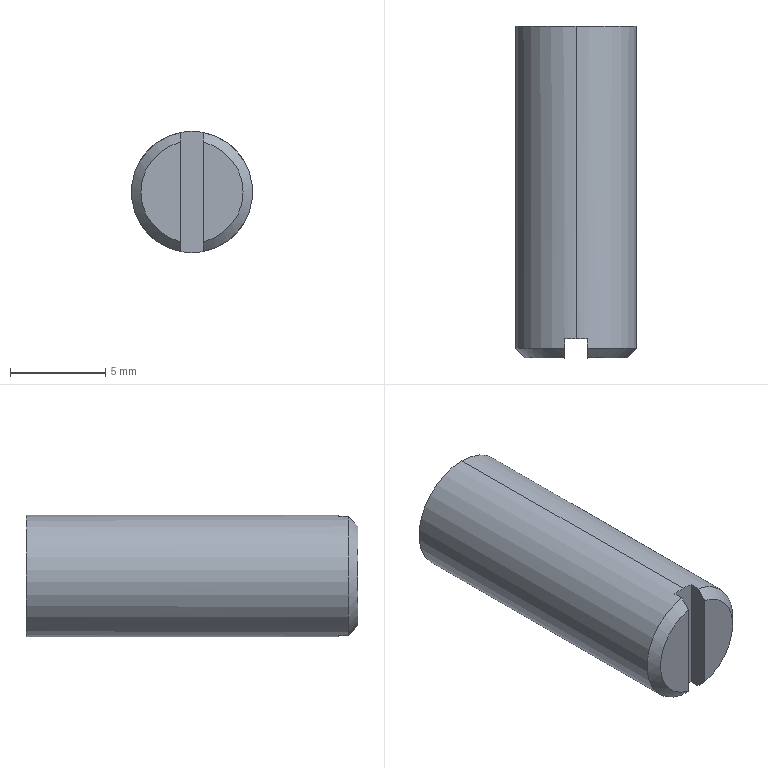Part | STEP file | 4-20.sldasm-Part-200 | 1 solid | 10 faces | box 6.35 x 17.375 x 6.35 mm | volume 540.618 mm3 | plane 6 | cylinder 2 | cone 2 | commonest cylinder face diameters 6.35 x2
STEP:
#1=CARTESIAN_POINT('',(-190.695,-588.425,-111.175));
#2=VERTEX_POINT('',#1);
#3=CARTESIAN_POINT('',(-190.695,-588.425,-104.825));
#4=VERTEX_POINT('',#3);
#5=CARTESIAN_POINT('',(-190.695,-588.425,-108.));
#6=DIRECTION('',(0.,-1.,0.));
#7=DIRECTION('',(0.,0.,-1.));
#8=AXIS2_PLACEMENT_3D('',#5,#6,#7);
#9=CIRCLE('',#8,3.175);
#10=EDGE_CURVE('',#2,#4,#9,.T.);
#11=ORIENTED_EDGE('',*,*,#10,.T.);
#12=CARTESIAN_POINT('',(-190.695,-604.8,-104.825));
#13=VERTEX_POINT('',#12);
#14=CARTESIAN_POINT('',(-190.695,-588.425,-104.825));
#15=DIRECTION('',(0.,-1.,0.));
#16=VECTOR('',#15,1000.);
#17=LINE('',#14,#16);
#18=EDGE_CURVE('',#4,#13,#17,.T.);
#19=ORIENTED_EDGE('',*,*,#18,.T.);
#20=CARTESIAN_POINT('',(-190.095,-604.8,-104.882));
#21=VERTEX_POINT('',#20);
#22=CARTESIAN_POINT('',(-190.695,-604.8,-108.));
#23=DIRECTION('',(0.,-1.,0.));
#24=DIRECTION('',(0.,0.,1.));
#25=AXIS2_PLACEMENT_3D('',#22,#23,#24);
#26=CIRCLE('',#25,3.175);
#27=EDGE_CURVE('',#21,#13,#26,.T.);
#28=ORIENTED_EDGE('',*,*,#27,.F.);
#29=CARTESIAN_POINT('',(-190.095,-605.3,-104.882));
#30=VERTEX_POINT('',#29);
#31=CARTESIAN_POINT('',(-190.095,-588.425,-104.882));
#32=DIRECTION('',(0.,1.,0.));
#33=VECTOR('',#32,1000.);
#34=LINE('',#31,#33);
#35=EDGE_CURVE('',#30,#21,#34,.T.);
#36=ORIENTED_EDGE('',*,*,#35,.F.);
#37=CARTESIAN_POINT('',(-190.095,-605.3,-111.118));
#38=VERTEX_POINT('',#37);
#39=CARTESIAN_POINT('',(-190.695,-605.3,-108.));
#40=DIRECTION('',(0.,1.,0.));
#41=DIRECTION('',(0.,0.,-1.));
#42=AXIS2_PLACEMENT_3D('',#39,#40,#41);
#43=CIRCLE('',#42,3.175);
#44=EDGE_CURVE('',#30,#38,#43,.T.);
#45=ORIENTED_EDGE('',*,*,#44,.T.);
#46=CARTESIAN_POINT('',(-190.095,-604.8,-111.118));
#47=VERTEX_POINT('',#46);
#48=CARTESIAN_POINT('',(-190.095,-588.425,-111.118));
#49=DIRECTION('',(0.,-1.,0.));
#50=VECTOR('',#49,1000.);
#51=LINE('',#48,#50);
#52=EDGE_CURVE('',#47,#38,#51,.T.);
#53=ORIENTED_EDGE('',*,*,#52,.F.);
#54=CARTESIAN_POINT('',(-190.695,-604.8,-111.175));
#55=VERTEX_POINT('',#54);
#56=CARTESIAN_POINT('',(-190.695,-604.8,-108.));
#57=DIRECTION('',(0.,-1.,0.));
#58=DIRECTION('',(0.,0.,1.));
#59=AXIS2_PLACEMENT_3D('',#56,#57,#58);
#60=CIRCLE('',#59,3.175);
#61=EDGE_CURVE('',#55,#47,#60,.T.);
#62=ORIENTED_EDGE('',*,*,#61,.F.);
#63=CARTESIAN_POINT('',(-190.695,-588.425,-111.175));
#64=DIRECTION('',(0.,-1.,0.));
#65=VECTOR('',#64,1000.);
#66=LINE('',#63,#65);
#67=EDGE_CURVE('',#2,#55,#66,.T.);
#68=ORIENTED_EDGE('',*,*,#67,.F.);
#69=EDGE_LOOP('',(#11,#19,#28,#36,#45,#53,#62,#68));
#70=FACE_OUTER_BOUND('',#69,.T.);
#71=CARTESIAN_POINT('',(-190.695,-588.425,-108.));
#72=DIRECTION('',(0.,-1.,0.));
#73=DIRECTION('',(0.,0.,-1.));
#74=AXIS2_PLACEMENT_3D('',#71,#72,#73);
#75=CYLINDRICAL_SURFACE('',#74,3.175);
#76=ADVANCED_FACE('',(#70),#75,.T.);
#77=CARTESIAN_POINT('',(-191.295,-605.8,-110.607));
#78=VERTEX_POINT('',#77);
#79=CARTESIAN_POINT('',(-191.295,-605.8,-105.393));
#80=VERTEX_POINT('',#79);
#81=CARTESIAN_POINT('',(-191.295,-605.8,-108.25));
#82=DIRECTION('',(0.,0.,1.));
#83=VECTOR('',#82,1000.);
#84=LINE('',#81,#83);
#85=EDGE_CURVE('',#78,#80,#84,.T.);
#86=ORIENTED_EDGE('',*,*,#85,.T.);
#87=CARTESIAN_POINT('',(-190.695,-605.8,-108.));
#88=DIRECTION('',(0.,-1.,0.));
#89=DIRECTION('',(0.,0.,-1.));
#90=AXIS2_PLACEMENT_3D('',#87,#88,#89);
#91=CIRCLE('',#90,2.675);
#92=EDGE_CURVE('',#80,#78,#91,.T.);
#93=ORIENTED_EDGE('',*,*,#92,.T.);
#94=EDGE_LOOP('',(#86,#93));
#95=FACE_OUTER_BOUND('',#94,.T.);
#96=CARTESIAN_POINT('',(-190.695,-605.8,-108.));
#97=DIRECTION('',(0.,-1.,0.));
#98=DIRECTION('',(0.,0.,-1.));
#99=AXIS2_PLACEMENT_3D('',#96,#97,#98);
#100=PLANE('',#99);
#101=ADVANCED_FACE('',(#95),#100,.T.);
#102=CARTESIAN_POINT('',(-190.095,-605.8,-105.393));
#103=VERTEX_POINT('',#102);
#104=CARTESIAN_POINT('',(-190.095,-605.8,-110.607));
#105=VERTEX_POINT('',#104);
#106=CARTESIAN_POINT('',(-190.095,-605.8,-108.25));
#107=DIRECTION('',(0.,0.,-1.));
#108=VECTOR('',#107,1000.);
#109=LINE('',#106,#108);
#110=EDGE_CURVE('',#103,#105,#109,.T.);
#111=ORIENTED_EDGE('',*,*,#110,.T.);
#112=CARTESIAN_POINT('',(-190.695,-605.8,-108.));
#113=DIRECTION('',(0.,-1.,0.));
#114=DIRECTION('',(0.,0.,-1.));
#115=AXIS2_PLACEMENT_3D('',#112,#113,#114);
#116=CIRCLE('',#115,2.675);
#117=EDGE_CURVE('',#105,#103,#116,.T.);
#118=ORIENTED_EDGE('',*,*,#117,.T.);
#119=EDGE_LOOP('',(#111,#118));
#120=FACE_OUTER_BOUND('',#119,.T.);
#121=CARTESIAN_POINT('',(-190.695,-605.8,-108.));
#122=DIRECTION('',(0.,-1.,0.));
#123=DIRECTION('',(0.,0.,-1.));
#124=AXIS2_PLACEMENT_3D('',#121,#122,#123);
#125=PLANE('',#124);
#126=ADVANCED_FACE('',(#120),#125,.T.);
#127=ORIENTED_EDGE('',*,*,#10,.F.);
#128=CARTESIAN_POINT('',(-190.695,-588.425,-108.));
#129=DIRECTION('',(0.,-1.,0.));
#130=DIRECTION('',(0.,0.,-1.));
#131=AXIS2_PLACEMENT_3D('',#128,#129,#130);
#132=CIRCLE('',#131,3.175);
#133=EDGE_CURVE('',#4,#2,#132,.T.);
#134=ORIENTED_EDGE('',*,*,#133,.F.);
#135=EDGE_LOOP('',(#127,#134));
#136=FACE_OUTER_BOUND('',#135,.T.);
#137=CARTESIAN_POINT('',(-190.695,-588.425,-108.));
#138=DIRECTION('',(0.,1.,0.));
#139=DIRECTION('',(0.,0.,1.));
#140=AXIS2_PLACEMENT_3D('',#137,#138,#139);
#141=PLANE('',#140);
#142=ADVANCED_FACE('',(#136),#141,.T.);
#143=ORIENTED_EDGE('',*,*,#18,.F.);
#144=ORIENTED_EDGE('',*,*,#133,.T.);
#145=ORIENTED_EDGE('',*,*,#67,.T.);
#146=CARTESIAN_POINT('',(-191.295,-604.8,-111.118));
#147=VERTEX_POINT('',#146);
#148=CARTESIAN_POINT('',(-190.695,-604.8,-108.));
#149=DIRECTION('',(0.,-1.,0.));
#150=DIRECTION('',(0.,0.,1.));
#151=AXIS2_PLACEMENT_3D('',#148,#149,#150);
#152=CIRCLE('',#151,3.175);
#153=EDGE_CURVE('',#147,#55,#152,.T.);
#154=ORIENTED_EDGE('',*,*,#153,.F.);
#155=CARTESIAN_POINT('',(-191.295,-605.3,-111.118));
#156=VERTEX_POINT('',#155);
#157=CARTESIAN_POINT('',(-191.295,-588.425,-111.118));
#158=DIRECTION('',(0.,1.,0.));
#159=VECTOR('',#158,1000.);
#160=LINE('',#157,#159);
#161=EDGE_CURVE('',#156,#147,#160,.T.);
#162=ORIENTED_EDGE('',*,*,#161,.F.);
#163=CARTESIAN_POINT('',(-191.295,-605.3,-104.882));
#164=VERTEX_POINT('',#163);
#165=CARTESIAN_POINT('',(-190.695,-605.3,-108.));
#166=DIRECTION('',(0.,1.,0.));
#167=DIRECTION('',(0.,0.,-1.));
#168=AXIS2_PLACEMENT_3D('',#165,#166,#167);
#169=CIRCLE('',#168,3.175);
#170=EDGE_CURVE('',#156,#164,#169,.T.);
#171=ORIENTED_EDGE('',*,*,#170,.T.);
#172=CARTESIAN_POINT('',(-191.295,-604.8,-104.882));
#173=VERTEX_POINT('',#172);
#174=CARTESIAN_POINT('',(-191.295,-588.425,-104.882));
#175=DIRECTION('',(0.,-1.,0.));
#176=VECTOR('',#175,1000.);
#177=LINE('',#174,#176);
#178=EDGE_CURVE('',#173,#164,#177,.T.);
#179=ORIENTED_EDGE('',*,*,#178,.F.);
#180=CARTESIAN_POINT('',(-190.695,-604.8,-108.));
#181=DIRECTION('',(0.,-1.,0.));
#182=DIRECTION('',(0.,0.,1.));
#183=AXIS2_PLACEMENT_3D('',#180,#181,#182);
#184=CIRCLE('',#183,3.175);
#185=EDGE_CURVE('',#13,#173,#184,.T.);
#186=ORIENTED_EDGE('',*,*,#185,.F.);
#187=EDGE_LOOP('',(#143,#144,#145,#154,#162,#171,#179,#186));
#188=FACE_OUTER_BOUND('',#187,.T.);
#189=CARTESIAN_POINT('',(-190.695,-588.425,-108.));
#190=DIRECTION('',(0.,-1.,0.));
#191=DIRECTION('',(0.,0.,-1.));
#192=AXIS2_PLACEMENT_3D('',#189,#190,#191);
#193=CYLINDRICAL_SURFACE('',#192,3.175);
#194=ADVANCED_FACE('',(#188),#193,.T.);
#195=ORIENTED_EDGE('',*,*,#178,.T.);
#196=CARTESIAN_POINT('',(-191.295,-605.3,-104.882));
#197=CARTESIAN_POINT('',(-191.295,-605.467,-105.052));
#198=CARTESIAN_POINT('',(-191.295,-605.634,-105.222));
#199=CARTESIAN_POINT('',(-191.295,-605.8,-105.393));
#200=B_SPLINE_CURVE_WITH_KNOTS('',3,(#196,#197,#198,#199),.UNSPECIFIED.,.F.,.F.,(4,4),(0.,0.0007149),.UNSPECIFIED.);
#201=EDGE_CURVE('',#164,#80,#200,.T.);
#202=ORIENTED_EDGE('',*,*,#201,.T.);
#203=ORIENTED_EDGE('',*,*,#85,.F.);
#204=CARTESIAN_POINT('',(-191.295,-605.8,-110.607));
#205=CARTESIAN_POINT('',(-191.295,-605.634,-110.778));
#206=CARTESIAN_POINT('',(-191.295,-605.467,-110.948));
#207=CARTESIAN_POINT('',(-191.295,-605.3,-111.118));
#208=B_SPLINE_CURVE_WITH_KNOTS('',3,(#204,#205,#206,#207),.UNSPECIFIED.,.F.,.F.,(4,4),(0.,0.0007149),.UNSPECIFIED.);
#209=EDGE_CURVE('',#78,#156,#208,.T.);
#210=ORIENTED_EDGE('',*,*,#209,.T.);
#211=ORIENTED_EDGE('',*,*,#161,.T.);
#212=CARTESIAN_POINT('',(-191.295,-604.8,-108.25));
#213=DIRECTION('',(0.,0.,-1.));
#214=VECTOR('',#213,1000.);
#215=LINE('',#212,#214);
#216=EDGE_CURVE('',#173,#147,#215,.T.);
#217=ORIENTED_EDGE('',*,*,#216,.F.);
#218=EDGE_LOOP('',(#195,#202,#203,#210,#211,#217));
#219=FACE_OUTER_BOUND('',#218,.T.);
#220=CARTESIAN_POINT('',(-191.295,-604.8,-108.25));
#221=DIRECTION('',(-1.,0.,0.));
#222=DIRECTION('',(0.,1.,0.));
#223=AXIS2_PLACEMENT_3D('',#220,#221,#222);
#224=PLANE('',#223);
#225=ADVANCED_FACE('',(#219),#224,.F.);
#226=ORIENTED_EDGE('',*,*,#52,.T.);
#227=CARTESIAN_POINT('',(-190.095,-605.3,-111.118));
#228=CARTESIAN_POINT('',(-190.095,-605.467,-110.948));
#229=CARTESIAN_POINT('',(-190.095,-605.634,-110.778));
#230=CARTESIAN_POINT('',(-190.095,-605.8,-110.607));
#231=B_SPLINE_CURVE_WITH_KNOTS('',3,(#227,#228,#229,#230),.UNSPECIFIED.,.F.,.F.,(4,4),(0.,0.0007149),.UNSPECIFIED.);
#232=EDGE_CURVE('',#38,#105,#231,.T.);
#233=ORIENTED_EDGE('',*,*,#232,.T.);
#234=ORIENTED_EDGE('',*,*,#110,.F.);
#235=CARTESIAN_POINT('',(-190.095,-605.8,-105.393));
#236=CARTESIAN_POINT('',(-190.095,-605.634,-105.222));
#237=CARTESIAN_POINT('',(-190.095,-605.467,-105.052));
#238=CARTESIAN_POINT('',(-190.095,-605.3,-104.882));
#239=B_SPLINE_CURVE_WITH_KNOTS('',3,(#235,#236,#237,#238),.UNSPECIFIED.,.F.,.F.,(4,4),(0.,0.0007149),.UNSPECIFIED.);
#240=EDGE_CURVE('',#103,#30,#239,.T.);
#241=ORIENTED_EDGE('',*,*,#240,.T.);
#242=ORIENTED_EDGE('',*,*,#35,.T.);
#243=CARTESIAN_POINT('',(-190.095,-604.8,-108.25));
#244=DIRECTION('',(0.,0.,1.));
#245=VECTOR('',#244,1000.);
#246=LINE('',#243,#245);
#247=EDGE_CURVE('',#47,#21,#246,.T.);
#248=ORIENTED_EDGE('',*,*,#247,.F.);
#249=EDGE_LOOP('',(#226,#233,#234,#241,#242,#248));
#250=FACE_OUTER_BOUND('',#249,.T.);
#251=CARTESIAN_POINT('',(-190.095,-604.8,-108.25));
#252=DIRECTION('',(1.,0.,0.));
#253=DIRECTION('',(0.,-1.,0.));
#254=AXIS2_PLACEMENT_3D('',#251,#252,#253);
#255=PLANE('',#254);
#256=ADVANCED_FACE('',(#250),#255,.F.);
#257=ORIENTED_EDGE('',*,*,#153,.T.);
#258=ORIENTED_EDGE('',*,*,#61,.T.);
#259=ORIENTED_EDGE('',*,*,#247,.T.);
#260=ORIENTED_EDGE('',*,*,#27,.T.);
#261=ORIENTED_EDGE('',*,*,#185,.T.);
#262=ORIENTED_EDGE('',*,*,#216,.T.);
#263=EDGE_LOOP('',(#257,#258,#259,#260,#261,#262));
#264=FACE_OUTER_BOUND('',#263,.T.);
#265=CARTESIAN_POINT('',(-190.695,-604.8,-108.25));
#266=DIRECTION('',(0.,1.,0.));
#267=DIRECTION('',(0.,0.,1.));
#268=AXIS2_PLACEMENT_3D('',#265,#266,#267);
#269=PLANE('',#268);
#270=ADVANCED_FACE('',(#264),#269,.F.);
#271=ORIENTED_EDGE('',*,*,#209,.F.);
#272=ORIENTED_EDGE('',*,*,#92,.F.);
#273=ORIENTED_EDGE('',*,*,#201,.F.);
#274=ORIENTED_EDGE('',*,*,#170,.F.);
#275=EDGE_LOOP('',(#271,#272,#273,#274));
#276=FACE_OUTER_BOUND('',#275,.T.);
#277=CARTESIAN_POINT('',(-190.695,-605.3,-108.));
#278=DIRECTION('',(0.,1.,0.));
#279=DIRECTION('',(0.,0.,1.));
#280=AXIS2_PLACEMENT_3D('',#277,#278,#279);
#281=CONICAL_SURFACE('',#280,3.175,0.7854);
#282=ADVANCED_FACE('',(#276),#281,.T.);
#283=ORIENTED_EDGE('',*,*,#240,.F.);
#284=ORIENTED_EDGE('',*,*,#117,.F.);
#285=ORIENTED_EDGE('',*,*,#232,.F.);
#286=ORIENTED_EDGE('',*,*,#44,.F.);
#287=EDGE_LOOP('',(#283,#284,#285,#286));
#288=FACE_OUTER_BOUND('',#287,.T.);
#289=CARTESIAN_POINT('',(-190.695,-605.3,-108.));
#290=DIRECTION('',(0.,1.,0.));
#291=DIRECTION('',(0.,0.,1.));
#292=AXIS2_PLACEMENT_3D('',#289,#290,#291);
#293=CONICAL_SURFACE('',#292,3.175,0.7854);
#294=ADVANCED_FACE('',(#288),#293,.T.);
#295=CLOSED_SHELL('',(#76,#101,#126,#142,#194,#225,#256,#270,#282,#294));
#296=MANIFOLD_SOLID_BREP('',#295);
#297=CARTESIAN_POINT('',(0.,0.,0.));
#298=DIRECTION('',(0.,0.,1.));
#299=DIRECTION('',(1.,0.,0.));
#300=AXIS2_PLACEMENT_3D('',#297,#298,#299);
#301=(LENGTH_UNIT()NAMED_UNIT(*)SI_UNIT(.MILLI.,.METRE.));
#302=UNCERTAINTY_MEASURE_WITH_UNIT(LENGTH_MEASURE(0.00001),#301,'','');
#303=(NAMED_UNIT(*)PLANE_ANGLE_UNIT()SI_UNIT($,.RADIAN.));
#304=(NAMED_UNIT(*)SI_UNIT($,.STERADIAN.)SOLID_ANGLE_UNIT());
#305=(GEOMETRIC_REPRESENTATION_CONTEXT(3)GLOBAL_UNCERTAINTY_ASSIGNED_CONTEXT((#302))GLOBAL_UNIT_ASSIGNED_CONTEXT((#301,#303,#304))REPRESENTATION_CONTEXT('',''));
#306=ADVANCED_BREP_SHAPE_REPRESENTATION('',(#296,#300),#305);